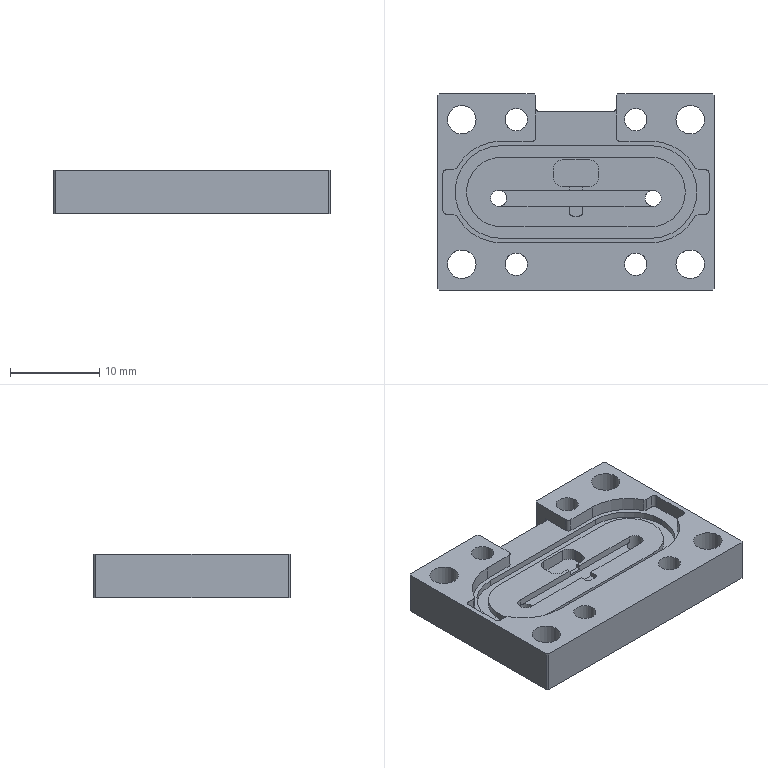NC program | NX | posted with a generic post | part box 31 x 22 x 4.9 mm
Lines 4624 to 5424 of 7945:
(PLANAR_MILL_2 , TOOL : 1C-4L-15L)
N9138 T05 M6
N9140 G54
N9142 G17 G0 G90 X-12.694 Y1.442 S4000 M3
N9144 G43 Z20. H5
N9146 Z-1.4
N9148 G94 G1 X-12.883 Y0.942 F300.
N9150 X-12.953 Y-0.5 Z-1.402
N9152 X-12.575 Y-1.893 Z-1.403
N9154 X-11.787 Y-3.102 Z-1.404
N9156 X-10.998 Y-3.798 Z-1.405
N9158 X-9.987 Y-4.331 Z-1.406
N9160 X-8.876 Y-4.6 Z-1.407
N9162 X8.876 Z-1.423
N9164 X9.987 Y-4.331 Z-1.424
N9166 X10.998 Y-3.798 Z-1.425
N9168 X11.787 Y-3.102 Z-1.426
N9170 X12.57 Y-1.905 Z-1.427
N9172 X12.95 Y-0.526 Z-1.428
N9174 Y0.526 Z-1.429
N9176 X12.645 Y1.728 Z-1.43
N9178 X12.033 Y2.806 Z-1.431
N9180 X11.156 Y3.683 Z-1.432
N9182 X10.078 Y4.295 Z-1.433
N9184 X8.876 Y4.6 Z-1.434
N9186 X-8.876 Z-1.45
N9188 X-10.267 Y4.214 Z-1.451
N9190 X-11.472 Y3.419 Z-1.452
N9192 X-12.373 Y2.292 Z-1.454
N9194 X-12.883 Y0.942 Z-1.455
N9196 X-12.953 Y-0.5 Z-1.456
N9198 X-12.575 Y-1.893 Z-1.457
N9200 X-11.787 Y-3.102 Z-1.459
N9202 X-10.998 Y-3.798 Z-1.46
N9204 X-9.987 Y-4.331 Z-1.461
N9206 X-8.876 Y-4.6 Z-1.462
N9208 X8.876 Z-1.477
N9210 X9.987 Y-4.331 Z-1.478
N9212 X10.998 Y-3.798 Z-1.479
N9214 X11.787 Y-3.102 Z-1.48
N9216 X12.57 Y-1.905 Z-1.481
N9218 X12.95 Y-0.526 Z-1.483
N9220 Y0.526
N9222 X12.645 Y1.728 Z-1.485
N9224 X12.033 Y2.806 Z-1.486
N9226 X11.156 Y3.683 Z-1.487
N9228 X10.078 Y4.295 Z-1.488
N9230 X8.876 Y4.6 Z-1.489
N9232 X-8.876 Z-1.504
N9234 X-10.267 Y4.214 Z-1.506
N9236 X-11.472 Y3.419 Z-1.507
N9238 X-12.373 Y2.292 Z-1.508
N9240 X-12.883 Y0.942 Z-1.509
N9242 X-12.953 Y-0.5 Z-1.511
N9244 X-12.575 Y-1.893 Z-1.512
N9246 X-11.787 Y-3.102 Z-1.513
N9248 X-10.998 Y-3.798 Z-1.514
N9250 X-9.987 Y-4.331 Z-1.515
N9252 X-8.876 Y-4.6 Z-1.516
N9254 X8.876 Z-1.532
N9256 X9.987 Y-4.331 Z-1.533
N9258 X10.998 Y-3.798 Z-1.534
N9260 X11.787 Y-3.102
N9262 X12.57 Y-1.905 Z-1.536
N9264 X12.95 Y-0.526 Z-1.537
N9266 Y0.526 Z-1.538
N9268 X12.645 Y1.728 Z-1.539
N9270 X12.033 Y2.806 Z-1.54
N9272 X11.156 Y3.683 Z-1.541
N9274 X10.078 Y4.295 Z-1.542
N9276 X8.876 Y4.6 Z-1.543
N9278 X-8.876 Z-1.559
N9280 X-10.267 Y4.214 Z-1.56
N9282 X-11.472 Y3.419 Z-1.561
N9284 X-12.373 Y2.292 Z-1.563
N9286 X-12.883 Y0.942 Z-1.564
N9288 X-12.953 Y-0.5 Z-1.565
N9290 X-12.575 Y-1.893 Z-1.566
N9292 X-11.787 Y-3.102 Z-1.568
N9294 X-10.998 Y-3.798 Z-1.569
N9296 X-9.987 Y-4.331 Z-1.57
N9298 X-8.876 Y-4.6 Z-1.571
N9300 X8.876 Z-1.586
N9302 X9.987 Y-4.331 Z-1.587
N9304 X10.998 Y-3.798 Z-1.588
N9306 X11.787 Y-3.102 Z-1.589
N9308 X12.57 Y-1.905 Z-1.59
N9310 X12.95 Y-0.526 Z-1.591
N9312 Y0.526 Z-1.592
N9314 X12.645 Y1.728 Z-1.593
N9316 X12.033 Y2.806 Z-1.594
N9318 X11.156 Y3.683 Z-1.596
N9320 X10.078 Y4.295 Z-1.597
N9322 X8.876 Y4.6 Z-1.598
N9324 X-8.876 Z-1.613
N9326 X-10.267 Y4.214 Z-1.614
N9328 X-11.472 Y3.419 Z-1.616
N9330 X-12.373 Y2.292 Z-1.617
N9332 X-12.883 Y0.942 Z-1.618
N9334 X-12.953 Y-0.5 Z-1.62
N9336 X-12.575 Y-1.893 Z-1.621
N9338 X-11.787 Y-3.102 Z-1.622
N9340 X-10.998 Y-3.798 Z-1.623
N9342 X-9.987 Y-4.331 Z-1.624
N9344 X-8.876 Y-4.6 Z-1.625
N9346 X8.876 Z-1.64
N9348 X9.987 Y-4.331 Z-1.641
N9350 X10.998 Y-3.798 Z-1.642
N9352 X11.787 Y-3.102 Z-1.643
N9354 X12.57 Y-1.905 Z-1.645
N9356 X12.95 Y-0.526 Z-1.646
N9358 Y0.526 Z-1.647
N9360 X12.645 Y1.728 Z-1.648
N9362 X12.033 Y2.806 Z-1.649
N9364 X11.156 Y3.683 Z-1.65
N9366 X10.078 Y4.295 Z-1.651
N9368 X8.876 Y4.6 Z-1.652
N9370 X-8.876 Z-1.668
N9372 X-10.267 Y4.214 Z-1.669
N9374 X-11.472 Y3.419 Z-1.67
N9376 X-12.373 Y2.292 Z-1.671
N9378 X-12.883 Y0.942 Z-1.673
N9380 X-12.953 Y-0.5 Z-1.674
N9382 X-12.575 Y-1.893 Z-1.675
N9384 X-11.787 Y-3.102 Z-1.677
N9386 X-10.998 Y-3.798
N9388 X-9.987 Y-4.331 Z-1.678
N9390 X-8.876 Y-4.6 Z-1.679
N9392 X8.876 Z-1.695
N9394 X9.987 Y-4.331 Z-1.696
N9396 X10.998 Y-3.798 Z-1.697
N9398 X11.787 Y-3.102 Z-1.698
N9400 X12.57 Y-1.905 Z-1.699
N9402 X12.95 Y-0.526 Z-1.7
N9404 Y0.526 Z-1.701
N9406 X12.645 Y1.728 Z-1.702
N9408 X12.033 Y2.806 Z-1.703
N9410 X11.156 Y3.683 Z-1.704
N9412 X10.078 Y4.295 Z-1.706
N9414 X8.876 Y4.6 Z-1.707
N9416 X-8.876 Z-1.722
N9418 X-10.267 Y4.214 Z-1.723
N9420 X-11.472 Y3.419 Z-1.725
N9422 X-12.373 Y2.292 Z-1.726
N9424 X-12.883 Y0.942 Z-1.727
N9426 X-12.953 Y-0.5 Z-1.728
N9428 X-12.575 Y-1.893 Z-1.73
N9430 X-11.787 Y-3.102 Z-1.731
N9432 X-10.998 Y-3.798 Z-1.732
N9434 X-9.987 Y-4.331 Z-1.733
N9436 X-8.876 Y-4.6 Z-1.734
N9438 X8.876 Z-1.749
N9440 X9.987 Y-4.331 Z-1.75
N9442 X10.998 Y-3.798 Z-1.751
N9444 X11.787 Y-3.102 Z-1.752
N9446 X12.57 Y-1.905 Z-1.754
N9448 X12.95 Y-0.526 Z-1.755
N9450 Y0.526 Z-1.756
N9452 X12.645 Y1.728 Z-1.757
N9454 X12.033 Y2.806 Z-1.758
N9456 X11.156 Y3.683 Z-1.759
N9458 X10.078 Y4.295 Z-1.76
N9460 X8.876 Y4.6 Z-1.761
N9462 X-8.876 Z-1.777
N9464 X-10.267 Y4.214 Z-1.778
N9466 X-11.472 Y3.419 Z-1.779
N9468 X-12.373 Y2.292 Z-1.78
N9470 X-12.883 Y0.942 Z-1.782
N9472 X-12.953 Y-0.5 Z-1.783
N9474 X-12.575 Y-1.893 Z-1.784
N9476 X-11.787 Y-3.102 Z-1.785
N9478 X-10.998 Y-3.798 Z-1.786
N9480 X-9.987 Y-4.331 Z-1.787
N9482 X-8.876 Y-4.6 Z-1.788
N9484 X8.876 Z-1.804
N9486 X9.987 Y-4.331 Z-1.805
N9488 X10.998 Y-3.798 Z-1.806
N9490 X11.787 Y-3.102 Z-1.807
N9492 X12.57 Y-1.905 Z-1.808
N9494 X12.95 Y-0.526 Z-1.809
N9496 Y0.526 Z-1.81
N9498 X12.645 Y1.728 Z-1.811
N9500 X12.033 Y2.806 Z-1.812
N9502 X11.156 Y3.683 Z-1.813
N9504 X10.078 Y4.295 Z-1.814
N9506 X8.876 Y4.6 Z-1.816
N9508 X-8.876 Z-1.831
N9510 X-10.267 Y4.214 Z-1.832
N9512 X-11.472 Y3.419 Z-1.834
N9514 X-12.373 Y2.292 Z-1.835
N9516 X-12.883 Y0.942 Z-1.836
N9518 X-12.953 Y-0.5 Z-1.837
N9520 X-12.575 Y-1.893 Z-1.839
N9522 X-11.787 Y-3.102 Z-1.84
N9524 X-10.998 Y-3.798 Z-1.841
N9526 X-9.987 Y-4.331 Z-1.842
N9528 X-8.876 Y-4.6 Z-1.843
N9530 X8.876 Z-1.858
N9532 X9.987 Y-4.331 Z-1.859
N9534 X10.998 Y-3.798 Z-1.86
N9536 X11.787 Y-3.102 Z-1.861
N9538 X12.57 Y-1.905 Z-1.862
N9540 X12.95 Y-0.526 Z-1.864
N9542 Y0.526 Z-1.865
N9544 X12.645 Y1.728 Z-1.866
N9546 X12.033 Y2.806 Z-1.867
N9548 X11.156 Y3.683 Z-1.868
N9550 X10.078 Y4.295 Z-1.869
N9552 X8.876 Y4.6 Z-1.87
N9554 X-8.876 Z-1.885
N9556 X-10.267 Y4.214 Z-1.887
N9558 X-11.472 Y3.419 Z-1.888
N9560 X-12.373 Y2.292 Z-1.889
N9562 X-12.883 Y0.942 Z-1.891
N9564 X-12.953 Y-0.5 Z-1.892
N9566 X-12.575 Y-1.893 Z-1.893
N9568 X-11.787 Y-3.102 Z-1.894
N9570 X-10.998 Y-3.798 Z-1.895
N9572 X-9.987 Y-4.331 Z-1.896
N9574 X-8.876 Y-4.6 Z-1.897
N9576 X8.876 Z-1.913
N9578 X9.987 Y-4.331 Z-1.914
N9580 X10.998 Y-3.798 Z-1.915
N9582 X11.787 Y-3.102 Z-1.916
N9584 X12.57 Y-1.905 Z-1.917
N9586 X12.95 Y-0.526 Z-1.918
N9588 Y0.526 Z-1.919
N9590 X12.645 Y1.728 Z-1.92
N9592 X12.033 Y2.806 Z-1.921
N9594 X11.156 Y3.683 Z-1.922
N9596 X10.078 Y4.295 Z-1.923
N9598 X8.876 Y4.6 Z-1.924
N9600 X-8.876 Z-1.94
N9602 X-10.267 Y4.214 Z-1.941
N9604 X-11.472 Y3.419 Z-1.942
N9606 X-12.373 Y2.292 Z-1.944
N9608 X-12.883 Y0.942 Z-1.945
N9610 X-12.953 Y-0.5 Z-1.946
N9612 X-12.575 Y-1.893 Z-1.947
N9614 X-11.787 Y-3.102 Z-1.949
N9616 X-10.998 Y-3.798 Z-1.95
N9618 X-9.987 Y-4.331 Z-1.951
N9620 X-8.876 Y-4.6 Z-1.952
N9622 X8.876 Z-1.967
N9624 X9.987 Y-4.331 Z-1.968
N9626 X10.998 Y-3.798 Z-1.969
N9628 X11.787 Y-3.102 Z-1.97
N9630 X12.57 Y-1.905 Z-1.971
N9632 X12.95 Y-0.526 Z-1.973
N9634 Y0.526
N9636 X12.645 Y1.728 Z-1.975
N9638 X12.033 Y2.806 Z-1.976
N9640 X11.156 Y3.683 Z-1.977
N9642 X10.078 Y4.295 Z-1.978
N9644 X8.876 Y4.6 Z-1.979
N9646 X-8.876 Z-1.994
N9648 X-10.267 Y4.214 Z-1.996
N9650 X-11.472 Y3.419 Z-1.997
N9652 X-12.373 Y2.292 Z-1.998
N9654 X-12.883 Y0.942 Z-1.999
N9656 X-12.953 Y-0.5 Z-2.001
N9658 X-12.575 Y-1.893 Z-2.002
N9660 X-11.787 Y-3.102 Z-2.003
N9662 X-10.998 Y-3.798 Z-2.004
N9664 X-9.987 Y-4.331 Z-2.005
N9666 X-8.876 Y-4.6 Z-2.006
N9668 X8.876 Z-2.022
N9670 X9.987 Y-4.331 Z-2.023
N9672 X10.998 Y-3.798 Z-2.024
N9674 X11.787 Y-3.102 Z-2.025
N9676 X12.57 Y-1.905 Z-2.026
N9678 X12.95 Y-0.526 Z-2.027
N9680 Y0.526 Z-2.028
N9682 X12.645 Y1.728 Z-2.029
N9684 X12.033 Y2.806 Z-2.03
N9686 X11.156 Y3.683 Z-2.031
N9688 X10.078 Y4.295 Z-2.032
N9690 X8.876 Y4.6 Z-2.033
N9692 X-8.876 Z-2.049
N9694 X-10.267 Y4.214 Z-2.05
N9696 X-11.472 Y3.419 Z-2.051
N9698 X-12.373 Y2.292 Z-2.053
N9700 X-12.883 Y0.942 Z-2.054
N9702 X-12.953 Y-0.5 Z-2.055
N9704 X-12.575 Y-1.893 Z-2.056
N9706 X-11.787 Y-3.102 Z-2.058
N9708 X-10.998 Y-3.798 Z-2.059
N9710 X-9.987 Y-4.331 Z-2.06
N9712 X-8.876 Y-4.6 Z-2.061
N9714 X8.876 Z-2.076
N9716 X9.987 Y-4.331 Z-2.077
N9718 X10.998 Y-3.798 Z-2.078
N9720 X11.787 Y-3.102 Z-2.079
N9722 X12.57 Y-1.905 Z-2.08
N9724 X12.95 Y-0.526 Z-2.081
N9726 Y0.526 Z-2.082
N9728 X12.645 Y1.728 Z-2.083
N9730 X12.033 Y2.806 Z-2.085
N9732 X11.156 Y3.683 Z-2.086
N9734 X10.078 Y4.295 Z-2.087
N9736 X8.876 Y4.6 Z-2.088
N9738 X-8.876 Z-2.103
N9740 X-10.267 Y4.214 Z-2.105
N9742 X-11.472 Y3.419 Z-2.106
N9744 X-12.373 Y2.292 Z-2.107
N9746 X-12.883 Y0.942 Z-2.108
N9748 X-12.953 Y-0.5 Z-2.11
N9750 X-12.575 Y-1.893 Z-2.111
N9752 X-11.787 Y-3.102 Z-2.112
N9754 X-10.998 Y-3.798 Z-2.113
N9756 X-9.987 Y-4.331 Z-2.114
N9758 X-8.876 Y-4.6 Z-2.115
N9760 X8.876 Z-2.131
N9762 X9.987 Y-4.331 Z-2.132
N9764 X10.998 Y-3.798 Z-2.133
N9766 X11.787 Y-3.102
N9768 X12.57 Y-1.905 Z-2.135
N9770 X12.95 Y-0.526 Z-2.136
N9772 Y0.526 Z-2.137
N9774 X12.645 Y1.728 Z-2.138
N9776 X12.033 Y2.806 Z-2.139
N9778 X11.156 Y3.683 Z-2.14
N9780 X10.078 Y4.295 Z-2.141
N9782 X8.876 Y4.6 Z-2.142
N9784 X0. Z-2.15
N9786 X-8.35
N9788 G3 X-12.95 Y0. R4.6
N9790 X-8.35 Y-4.6 R4.6
N9792 G1 X8.35
N9794 G3 X12.95 Y0. R4.6
N9796 X8.35 Y4.6 R4.6
N9798 G1 X0.
N9800 Z-2.05
N9802 G0 Z20.
(PLANAR_MILL_2_COPY , TOOL : 1C-4L-15L)
N9804 X-0.15 Y-0.197
N9806 Z-1.4
N9808 G1 Y-2.1 Z-1.402
N9810 X0.15
N9812 Y1.2 Z-1.405
N9814 X-0.15
N9816 Y-2.1 Z-1.408
N9818 X0.15
N9820 Y1.2 Z-1.411
N9822 X-0.15
N9824 Y-2.1 Z-1.414
N9826 X0.15
N9828 Y1.2 Z-1.417
N9830 X-0.15 Z-1.418
N9832 Y-2.1 Z-1.421
N9834 X0.15
N9836 Y1.2 Z-1.424
N9838 X-0.15
N9840 Y-2.1 Z-1.427
N9842 X0.15
N9844 Y1.2 Z-1.43
N9846 X-0.15
N9848 Y-2.1 Z-1.433
N9850 X0.15
N9852 Y1.2 Z-1.436
N9854 X-0.15
N9856 Y-2.1 Z-1.439
N9858 X0.15 Z-1.44
N9860 Y1.2 Z-1.443
N9862 X-0.15
N9864 Y-2.1 Z-1.446
N9866 X0.15
N9868 Y1.2 Z-1.449
N9870 X-0.15
N9872 Y-2.1 Z-1.452
N9874 X0.15
N9876 Y1.2 Z-1.455
N9878 X-0.15
N9880 Y-2.1 Z-1.458
N9882 X0.15
N9884 Y1.2 Z-1.461
N9886 X-0.15 Z-1.462
N9888 Y-2.1 Z-1.464
N9890 X0.15 Z-1.465
N9892 Y1.2 Z-1.468
N9894 X-0.15
N9896 Y-2.1 Z-1.471
N9898 X0.15
N9900 Y1.2 Z-1.474
N9902 X-0.15
N9904 Y-2.1 Z-1.477
N9906 X0.15
N9908 Y1.2 Z-1.48
N9910 X-0.15
N9912 Y-2.1 Z-1.483
N9914 X0.15 Z-1.484
N9916 Y1.2 Z-1.486
N9918 X-0.15 Z-1.487
N9920 Y-2.1 Z-1.49
N9922 X0.15
N9924 Y1.2 Z-1.493
N9926 X-0.15
N9928 Y-2.1 Z-1.496
N9930 X0.15
N9932 Y1.2 Z-1.499
N9934 X-0.15
N9936 Y-2.1 Z-1.502
N9938 X0.15
N9940 Y1.2 Z-1.505
N9942 X-0.15 Z-1.506
N9944 Y-2.1 Z-1.508
N9946 X0.15 Z-1.509
N9948 Y1.2 Z-1.512
N9950 X-0.15
N9952 Y-2.1 Z-1.515
N9954 X0.15
N9956 Y1.2 Z-1.518
N9958 X-0.15
N9960 Y-2.1 Z-1.521
N9962 X0.15
N9964 Y1.2 Z-1.524
N9966 X-0.15
N9968 Y-2.1 Z-1.527
N9970 X0.15 Z-1.528
N9972 Y1.2 Z-1.53
N9974 X-0.15 Z-1.531
N9976 Y-2.1 Z-1.534
N9978 X0.15
N9980 Y1.2 Z-1.537
N9982 X-0.15
N9984 Y-2.1 Z-1.54
N9986 X0.15
N9988 Y1.2 Z-1.543
N9990 X-0.15
N9992 Y-2.1 Z-1.546
N9994 X0.15
N9996 Y1.2 Z-1.549
N9998 X-0.15 Z-1.55
N10000 Y-2.1 Z-1.552
N10002 X0.15 Z-1.553
N10004 Y1.2 Z-1.556
N10006 X-0.15
N10008 Y-2.1 Z-1.559
N10010 X0.15
N10012 Y1.2 Z-1.562
N10014 X-0.15
N10016 Y-2.1 Z-1.565
N10018 X0.15
N10020 Y1.2 Z-1.568
N10022 X-0.15
N10024 Y-2.1 Z-1.571
N10026 X0.15 Z-1.572
N10028 Y1.2 Z-1.574
N10030 X-0.15 Z-1.575
N10032 Y-2.1 Z-1.578
N10034 X0.15
N10036 Y1.2 Z-1.581
N10038 X-0.15
N10040 Y-2.1 Z-1.584
N10042 X0.15
N10044 Y1.2 Z-1.587
N10046 X-0.15
N10048 Y-2.1 Z-1.59
N10050 X0.15
N10052 Y1.2 Z-1.593
N10054 X-0.15 Z-1.594
N10056 Y-2.1 Z-1.596
N10058 X0.15 Z-1.597
N10060 Y1.2 Z-1.6
N10062 X-0.15
N10064 Y-2.1 Z-1.603
N10066 X0.15
N10068 Y1.2 Z-1.606
N10070 X-0.15
N10072 Y-2.1 Z-1.609
N10074 X0.15
N10076 Y1.2 Z-1.612
N10078 X-0.15
N10080 Y-2.1 Z-1.615
N10082 X0.15 Z-1.616
N10084 Y1.2 Z-1.618
N10086 X-0.15 Z-1.619
N10088 Y-2.1 Z-1.622
N10090 X0.15
N10092 Y1.2 Z-1.625
N10094 X-0.15
N10096 Y-2.1 Z-1.628
N10098 X0.15
N10100 Y1.2 Z-1.631
N10102 X-0.15
N10104 Y-2.1 Z-1.634
N10106 X0.15
N10108 Y1.2 Z-1.637
N10110 X-0.15 Z-1.638
N10112 Y-2.1 Z-1.64
N10114 X0.15 Z-1.641
N10116 Y1.2 Z-1.644
N10118 X-0.15
N10120 Y-2.1 Z-1.647
N10122 X0.15
N10124 Y1.2 Z-1.65
N10126 X-0.15
N10128 Y-2.1 Z-1.653
N10130 X0.15
N10132 Y1.2 Z-1.656
N10134 X-0.15
N10136 Y-2.1 Z-1.659
N10138 X0.15 Z-1.66
N10140 Y1.2 Z-1.662
N10142 X-0.15 Z-1.663
N10144 Y-2.1 Z-1.666
N10146 X0.15
N10148 Y1.2 Z-1.669
N10150 X-0.15
N10152 Y-2.1 Z-1.672
N10154 X0.15
N10156 Y1.2 Z-1.675
N10158 X-0.15
N10160 Y-2.1 Z-1.678
N10162 X0.15
N10164 Y1.2 Z-1.681
N10166 X-0.15 Z-1.682
N10168 Y-2.1 Z-1.684
N10170 X0.15 Z-1.685
N10172 Y1.2 Z-1.688
N10174 X-0.15
N10176 Y-2.1 Z-1.691
N10178 X0.15
N10180 Y1.2 Z-1.694
N10182 X-0.15
N10184 Y-2.1 Z-1.697
N10186 X0.15
N10188 Y1.2 Z-1.7
N10190 X-0.15
N10192 Y-2.1 Z-1.703
N10194 X0.15 Z-1.704
N10196 Y1.2 Z-1.706
N10198 X-0.15 Z-1.707
N10200 Y-2.1 Z-1.71
N10202 X0.15
N10204 Y1.2 Z-1.713
N10206 X-0.15
N10208 Y-2.1 Z-1.716
N10210 X0.15
N10212 Y1.2 Z-1.719
N10214 X-0.15
N10216 Y-2.1 Z-1.722
N10218 X0.15
N10220 Y1.2 Z-1.725
N10222 X-0.15 Z-1.726
N10224 Y-2.1 Z-1.728
N10226 X0.15 Z-1.729
N10228 Y1.2 Z-1.732
N10230 X-0.15
N10232 Y-2.1 Z-1.735
N10234 X0.15
N10236 Y1.2 Z-1.738
N10238 X-0.15
N10240 Y-2.1 Z-1.741
N10242 X0.15
N10244 Y1.2 Z-1.744
N10246 X-0.15
N10248 Y-2.1 Z-1.747
N10250 X0.15
N10252 Y1.2 Z-1.75
N10254 X-0.15 Z-1.751
N10256 Y-2.1 Z-1.754
N10258 X0.15
N10260 Y1.2 Z-1.757
N10262 X-0.15
N10264 Y-2.1 Z-1.76
N10266 X0.15
N10268 Y1.2 Z-1.763
N10270 X-0.15
N10272 Y-2.1 Z-1.766
N10274 X0.15
N10276 Y1.2 Z-1.769
N10278 X-0.15
N10280 Y-2.1 Z-1.772
N10282 X0.15 Z-1.773
N10284 Y1.2 Z-1.776
N10286 X-0.15
N10288 Y-2.1 Z-1.779
N10290 X0.15
N10292 Y1.2 Z-1.782
N10294 X-0.15
N10296 Y-2.1 Z-1.785
N10298 X0.15
N10300 Y1.2 Z-1.788
N10302 X-0.15
N10304 Y-2.1 Z-1.791
N10306 X0.15
N10308 Y1.2 Z-1.794
N10310 X-0.15 Z-1.795
N10312 Y-2.1 Z-1.798
N10314 X0.15
N10316 Y1.2 Z-1.801
N10318 X-0.15
N10320 Y-2.1 Z-1.804
N10322 X0.15
N10324 Y1.2 Z-1.807
N10326 X-0.15
N10328 Y-2.1 Z-1.81
N10330 X0.15
N10332 Y1.2 Z-1.813
N10334 X-0.15
N10336 Y-2.1 Z-1.816
N10338 X0.15 Z-1.817
N10340 Y1.2 Z-1.819
N10342 X-0.15 Z-1.82
N10344 Y-2.1 Z-1.823
N10346 X0.15
N10348 Y1.2 Z-1.826
N10350 X-0.15
N10352 Y-2.1 Z-1.829
N10354 X0.15
N10356 Y1.2 Z-1.832
N10358 X-0.15
N10360 Y-2.1 Z-1.835
N10362 X0.15
N10364 Y1.2 Z-1.838
N10366 X-0.15 Z-1.839
N10368 Y-2.1 Z-1.841
N10370 X0.15 Z-1.842
N10372 Y1.2 Z-1.845
N10374 X-0.15
N10376 Y-2.1 Z-1.848
N10378 X0.15
N10380 Y1.2 Z-1.851
N10382 X-0.15
N10384 Y-2.1 Z-1.854
N10386 X0.15
N10388 Y1.2 Z-1.857
N10390 X-0.15
N10392 Y-2.1 Z-1.86
N10394 X0.15 Z-1.861
N10396 Y1.2 Z-1.863
N10398 X-0.15 Z-1.864
N10400 Y-2.1 Z-1.867
N10402 X0.15
N10404 Y1.2 Z-1.87
N10406 X-0.15
N10408 Y-2.1 Z-1.873
N10410 X0.15
N10412 Y1.2 Z-1.876
N10414 X-0.15
N10416 Y-2.1 Z-1.879
N10418 X0.15
N10420 Y1.2 Z-1.882
N10422 X-0.15 Z-1.883
N10424 Y-2.1 Z-1.885
N10426 X0.15 Z-1.886
N10428 Y1.2 Z-1.889
N10430 X-0.15
N10432 Y-2.1 Z-1.892
N10434 X0.15
N10436 Y1.2 Z-1.895
N10438 X-0.15
N10440 Y-2.1 Z-1.898
N10442 X0.15
N10444 Y1.2 Z-1.901
N10446 X-0.15
N10448 Y-2.1 Z-1.904
N10450 X0.15 Z-1.905
N10452 Y1.2 Z-1.907
N10454 X-0.15 Z-1.908
N10456 Y-2.1 Z-1.911
N10458 X0.15
N10460 Y1.2 Z-1.914
N10462 X-0.15
N10464 Y-2.1 Z-1.917
N10466 X0.15
N10468 Y1.2 Z-1.92
N10470 X-0.15
N10472 Y-2.1 Z-1.923
N10474 X0.15
N10476 Y1.2 Z-1.926
N10478 X-0.15 Z-1.927
N10480 Y-2.1 Z-1.929
N10482 X0.15 Z-1.93
N10484 Y1.2 Z-1.933
N10486 X-0.15
N10488 Y-2.1 Z-1.936
N10490 X0.15
N10492 Y1.2 Z-1.939
N10494 X-0.15
N10496 Y-2.1 Z-1.942
N10498 X0.15
N10500 Y1.2 Z-1.945
N10502 X-0.15
N10504 Y-2.1 Z-1.948
N10506 X0.15 Z-1.949
N10508 Y-0.45 Z-1.95
N10510 Y1.2
N10512 X-0.15
N10514 Y-2.1
N10516 X0.15
N10518 Y-0.45
N10520 Z-1.85
N10522 G0 Z20.
N10524 M5
(FACE_MILLING_2_COPY , TOOL : 4J-10L-25L)
N10526 T16 M6
N10528 G54
N10530 G17 G0 G90 X0. Y13. S3000 M3
N10532 G43 Z20. H16
N10534 Z1.5
N10536 G94 G1 Z-1.5 F300.
N10538 Y11.
N10540 X2.48
N10542 G3 X2.47 Y10.8 R2.03
N10544 G1 Y6.1
N10546 G3 X4.9 Y3.67 R2.43
N10548 G1 X8.35
N10550 G2 X11.592 Y1.719 R3.67
N10552 G3 X12.339 Y0.931 R2.03
N10554 G1 X12.622 Y0.761
N10556 G3 X12.87 Y0.634 R2.03
N10558 G1 Y-0.634
N10560 G3 X12.622 Y-0.761 R2.03
N10562 G1 X12.339 Y-0.931
N10564 G3 X11.592 Y-1.719 R2.03
N10566 G2 X8.35 Y-3.67 R3.67
N10568 G1 X-8.35
N10570 G2 X-11.592 Y-1.719 R3.67
N10572 G3 X-12.339 Y-0.931 R2.03
N10574 G1 X-12.622 Y-0.761
N10576 G3 X-12.87 Y-0.634 R2.03
N10578 G1 Y0.634
N10580 G3 X-12.622 Y0.761 R2.03
N10582 G1 X-12.339 Y0.931
N10584 G3 X-11.592 Y1.719 R2.03
N10586 G2 X-8.35 Y3.67 R3.67
N10588 G1 X-4.9
N10590 G3 X-2.47 Y6.1 R2.43
N10592 G1 Y10.8
N10594 G3 X-2.48 Y11. R2.03
N10596 G1 X0.
N10598 Y4.964
N10600 G3 X4.9 Y1.07 R5.03
N10602 G1 X8.35
N10604 G2 X9.295 Y0.501 R1.07
N10606 G3 X9.603 Y0. R4.63
N10608 X9.295 Y-0.501 R4.63
N10610 G2 X8.35 Y-1.07 R1.07
N10612 G1 X-8.35
N10614 G2 X-9.295 Y-0.501 R1.07
N10616 G3 X-9.603 Y0. R4.63
N10618 X-9.295 Y0.501 R4.63
N10620 G2 X-8.35 Y1.07 R1.07
N10622 G1 X-4.9
N10624 G3 X0. Y4.964 R5.03
N10626 G1 Y1.342
N10628 G3 X0.68 Y0.73 R6.83
N10630 G1 X-0.68
N10632 G3 X0. Y1.342 R6.83
N10634 G1 X-1.435 Y2.735
N10636 Z1.5
N10638 G0 Z20.
(FACE_MILLING_2_COPY_COPY , TOOL : 4J-10L-25L)
N10640 X-2.835 Y14.763
N10642 Z1.5
N10644 G1 Z-1.5
N10646 G41 X-2.85 Y14.564 D16
N10648 X-2.495 Y11.
N10650 G2 X-2.485 Y10.8 R2.015
N10652 G1 Y6.1
N10654 G2 X-4.9 Y3.685 R2.415
N10656 G1 X-8.35
N10658 G3 X-11.606 Y1.726 R3.685
N10660 G2 X-12.347 Y0.944 R2.015
N10662 G1 X-12.63 Y0.773
N10664 G2 X-12.885 Y0.644 R2.015
N10666 G1 Y-0.644
N10668 G2 X-12.63 Y-0.773 R2.015
N10670 G1 X-12.347 Y-0.944
N10672 G2 X-11.606 Y-1.726 R2.015
N10674 G3 X-8.35 Y-3.685 R3.685
N10676 G1 X8.35
N10678 G3 X11.606 Y-1.726 R3.685
N10680 G2 X12.347 Y-0.944 R2.015
N10682 G1 X12.63 Y-0.773
N10684 G2 X12.885 Y-0.644 R2.015
N10686 G1 Y0.644
N10688 G2 X12.63 Y0.773 R2.015
N10690 G1 X12.347 Y0.944
N10692 G2 X11.606 Y1.726 R2.015
N10694 G3 X8.35 Y3.685 R3.685
N10696 G1 X4.9
N10698 G2 X2.485 Y6.1 R2.415
N10700 G1 Y10.8
N10702 G2 X2.495 Y11. R2.015
N10704 G1 X2.85 Y14.564
N10706 G40
N10708 X2.835 Y14.763
N10710 Z1.5
N10712 G0 Z20.
N10714 M5